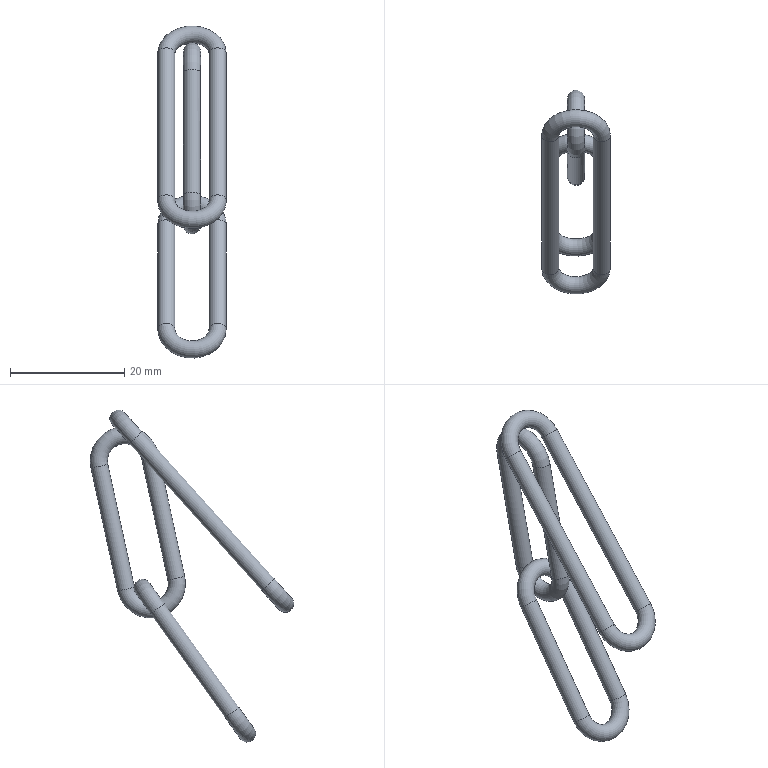Part | NX | features ACO1606-1-04.3 2 | 1 solid | 12 faces | box 12 x 35.608 x 58.107 mm | volume 1716 mm3 | torus 6 | cylinder 6 | commonest cylinder face diameters 3 x6
STEP:
#1=CARTESIAN_POINT('',(858.667,881.956,-129.86));
#2=VERTEX_POINT('',#1);
#3=CARTESIAN_POINT('',(860.167,881.956,-129.86));
#4=DIRECTION('',(0.,0.5837,0.812));
#5=DIRECTION('',(-1.,0.,0.));
#6=AXIS2_PLACEMENT_3D('',#3,#4,#5);
#7=CIRCLE('',#6,1.5);
#8=EDGE_CURVE('',#2,#2,#7,.T.);
#9=ORIENTED_EDGE('',*,*,#8,.T.);
#10=EDGE_LOOP('',(#9));
#11=FACE_BOUND('',#10,.T.);
#12=CARTESIAN_POINT('',(867.667,881.956,-129.86));
#13=VERTEX_POINT('',#12);
#14=CARTESIAN_POINT('',(869.167,881.956,-129.86));
#15=DIRECTION('',(0.,-0.5837,-0.812));
#16=DIRECTION('',(-1.,0.,0.));
#17=AXIS2_PLACEMENT_3D('',#14,#15,#16);
#18=CIRCLE('',#17,1.5);
#19=EDGE_CURVE('',#13,#13,#18,.T.);
#20=ORIENTED_EDGE('',*,*,#19,.F.);
#21=EDGE_LOOP('',(#20));
#22=FACE_BOUND('',#21,.T.);
#23=CARTESIAN_POINT('',(864.161,886.066,-126.148));
#24=VERTEX_POINT('',#23);
#25=CARTESIAN_POINT('',(865.173,886.066,-126.148));
#26=VERTEX_POINT('',#25);
#27=CARTESIAN_POINT('',(864.161,886.066,-126.148));
#28=CARTESIAN_POINT('',(863.968,886.07,-126.457));
#29=CARTESIAN_POINT('',(863.879,885.934,-127.03));
#30=CARTESIAN_POINT('',(864.124,885.389,-127.515));
#31=CARTESIAN_POINT('',(864.664,885.138,-127.587));
#32=CARTESIAN_POINT('',(865.206,885.384,-127.517));
#33=CARTESIAN_POINT('',(865.456,885.931,-127.036));
#34=CARTESIAN_POINT('',(865.366,886.07,-126.457));
#35=CARTESIAN_POINT('',(865.173,886.066,-126.148));
#36=B_SPLINE_CURVE_WITH_KNOTS('',3,(#27,#28,#29,#30,#31,#32,#33,#34,#35),.UNSPECIFIED.,.F.,.F.,(4,1,1,1,1,1,4),(-0.002168,-0.001085,-0.000544,-0.0000027,0.0005386,0.00108,0.002162),.UNSPECIFIED.);
#37=EDGE_CURVE('',#24,#26,#36,.T.);
#38=ORIENTED_EDGE('',*,*,#37,.T.);
#39=CARTESIAN_POINT('',(865.173,886.066,-126.148));
#40=CARTESIAN_POINT('',(865.064,886.064,-125.974));
#41=CARTESIAN_POINT('',(864.667,886.016,-125.734));
#42=CARTESIAN_POINT('',(864.27,886.064,-125.974));
#43=CARTESIAN_POINT('',(864.161,886.066,-126.148));
#44=B_SPLINE_CURVE_WITH_KNOTS('',3,(#39,#40,#41,#42,#43),.UNSPECIFIED.,.F.,.F.,(4,1,4),(-0.0006085,-0.000000009,0.0006085),.UNSPECIFIED.);
#45=EDGE_CURVE('',#26,#24,#44,.T.);
#46=ORIENTED_EDGE('',*,*,#45,.T.);
#47=EDGE_LOOP('',(#38,#46));
#48=FACE_BOUND('',#47,.T.);
#49=CARTESIAN_POINT('',(864.667,881.956,-129.86));
#50=DIRECTION('',(0.,0.812,-0.5837));
#51=DIRECTION('',(0.,0.5837,0.812));
#52=AXIS2_PLACEMENT_3D('',#49,#50,#51);
#53=TOROIDAL_SURFACE('',#52,4.5,1.5);
#54=ADVANCED_FACE('',(#11,#22,#48),#53,.T.);
#55=CARTESIAN_POINT('',(867.667,868.886,-148.041));
#56=VERTEX_POINT('',#55);
#57=CARTESIAN_POINT('',(869.167,868.886,-148.041));
#58=DIRECTION('',(0.,-0.5837,-0.812));
#59=DIRECTION('',(-1.,0.,0.));
#60=AXIS2_PLACEMENT_3D('',#57,#58,#59);
#61=CIRCLE('',#60,1.5);
#62=EDGE_CURVE('',#56,#56,#61,.T.);
#63=ORIENTED_EDGE('',*,*,#62,.F.);
#64=EDGE_LOOP('',(#63));
#65=FACE_BOUND('',#64,.T.);
#66=ORIENTED_EDGE('',*,*,#19,.T.);
#67=EDGE_LOOP('',(#66));
#68=FACE_BOUND('',#67,.T.);
#69=CARTESIAN_POINT('',(869.167,875.421,-138.951));
#70=DIRECTION('',(0.,0.5837,0.812));
#71=DIRECTION('',(0.,-0.812,0.5837));
#72=AXIS2_PLACEMENT_3D('',#69,#70,#71);
#73=CYLINDRICAL_SURFACE('',#72,1.5);
#74=ADVANCED_FACE('',(#65,#68),#73,.T.);
#75=ORIENTED_EDGE('',*,*,#62,.T.);
#76=EDGE_LOOP('',(#75));
#77=FACE_BOUND('',#76,.T.);
#78=CARTESIAN_POINT('',(858.667,868.886,-148.041));
#79=VERTEX_POINT('',#78);
#80=CARTESIAN_POINT('',(860.167,868.886,-148.041));
#81=DIRECTION('',(0.,0.5837,0.812));
#82=DIRECTION('',(-1.,0.,0.));
#83=AXIS2_PLACEMENT_3D('',#80,#81,#82);
#84=CIRCLE('',#83,1.5);
#85=EDGE_CURVE('',#79,#79,#84,.T.);
#86=ORIENTED_EDGE('',*,*,#85,.F.);
#87=EDGE_LOOP('',(#86));
#88=FACE_BOUND('',#87,.T.);
#89=CARTESIAN_POINT('',(864.667,868.886,-148.041));
#90=DIRECTION('',(0.,0.812,-0.5837));
#91=DIRECTION('',(0.,0.5837,0.812));
#92=AXIS2_PLACEMENT_3D('',#89,#90,#91);
#93=TOROIDAL_SURFACE('',#92,4.5,1.5);
#94=ADVANCED_FACE('',(#77,#88),#93,.T.);
#95=ORIENTED_EDGE('',*,*,#8,.F.);
#96=EDGE_LOOP('',(#95));
#97=FACE_BOUND('',#96,.T.);
#98=ORIENTED_EDGE('',*,*,#85,.T.);
#99=EDGE_LOOP('',(#98));
#100=FACE_BOUND('',#99,.T.);
#101=CARTESIAN_POINT('',(860.167,875.421,-138.951));
#102=DIRECTION('',(0.,-0.5837,-0.812));
#103=DIRECTION('',(0.,0.812,-0.5837));
#104=AXIS2_PLACEMENT_3D('',#101,#102,#103);
#105=CYLINDRICAL_SURFACE('',#104,1.5);
#106=ADVANCED_FACE('',(#97,#100),#105,.T.);
#107=CARTESIAN_POINT('',(867.667,885.762,-99.932));
#108=VERTEX_POINT('',#107);
#109=CARTESIAN_POINT('',(869.167,885.762,-99.932));
#110=DIRECTION('',(0.,0.6691,0.7431));
#111=DIRECTION('',(-1.,0.,0.));
#112=AXIS2_PLACEMENT_3D('',#109,#110,#111);
#113=CIRCLE('',#112,1.5);
#114=EDGE_CURVE('',#108,#108,#113,.T.);
#115=ORIENTED_EDGE('',*,*,#114,.T.);
#116=EDGE_LOOP('',(#115));
#117=FACE_BOUND('',#116,.T.);
#118=CARTESIAN_POINT('',(858.667,885.762,-99.932));
#119=VERTEX_POINT('',#118);
#120=CARTESIAN_POINT('',(860.167,885.762,-99.932));
#121=DIRECTION('',(0.,-0.6691,-0.7431));
#122=DIRECTION('',(-1.,0.,0.));
#123=AXIS2_PLACEMENT_3D('',#120,#121,#122);
#124=CIRCLE('',#123,1.5);
#125=EDGE_CURVE('',#119,#119,#124,.T.);
#126=ORIENTED_EDGE('',*,*,#125,.F.);
#127=EDGE_LOOP('',(#126));
#128=FACE_BOUND('',#127,.T.);
#129=CARTESIAN_POINT('',(864.667,888.765,-98.088));
#130=VERTEX_POINT('',#129);
#131=CARTESIAN_POINT('',(864.226,888.545,-98.107));
#132=CARTESIAN_POINT('',(864.667,888.875,-98.078));
#133=CARTESIAN_POINT('',(865.107,888.547,-98.108));
#134=CARTESIAN_POINT('',(864.668,888.259,-97.989));
#135=CARTESIAN_POINT('',(864.226,888.545,-98.107));
#136=CARTESIAN_POINT('',(864.667,888.875,-98.078));
#137=CARTESIAN_POINT('',(865.107,888.547,-98.108));
#138=B_SPLINE_CURVE_WITH_KNOTS('',3,(#131,#132,#133,#134,#135,#136,#137),.UNSPECIFIED.,.T.,.F.,(1,1,1,1,1,1,1,1,1,1,1),(-0.001184,-0.0007892,-0.0003946,0.,0.0003946,0.0007892,0.001184,0.001578,0.001973,0.002368,0.002762),.UNSPECIFIED.);
#139=EDGE_CURVE('',#130,#130,#138,.T.);
#140=ORIENTED_EDGE('',*,*,#139,.F.);
#141=EDGE_LOOP('',(#140));
#142=FACE_BOUND('',#141,.T.);
#143=CARTESIAN_POINT('',(864.667,885.762,-99.932));
#144=DIRECTION('',(0.,-0.7431,0.6691));
#145=DIRECTION('',(0.,-0.6691,-0.7431));
#146=AXIS2_PLACEMENT_3D('',#143,#144,#145);
#147=TOROIDAL_SURFACE('',#146,4.5,1.5);
#148=ADVANCED_FACE('',(#117,#128,#142),#147,.T.);
#149=CARTESIAN_POINT('',(858.667,862.604,-125.651));
#150=VERTEX_POINT('',#149);
#151=CARTESIAN_POINT('',(860.167,862.604,-125.651));
#152=DIRECTION('',(0.,-0.6691,-0.7431));
#153=DIRECTION('',(-1.,0.,0.));
#154=AXIS2_PLACEMENT_3D('',#151,#152,#153);
#155=CIRCLE('',#154,1.5);
#156=EDGE_CURVE('',#150,#150,#155,.T.);
#157=ORIENTED_EDGE('',*,*,#156,.F.);
#158=EDGE_LOOP('',(#157));
#159=FACE_BOUND('',#158,.T.);
#160=ORIENTED_EDGE('',*,*,#125,.T.);
#161=EDGE_LOOP('',(#160));
#162=FACE_BOUND('',#161,.T.);
#163=CARTESIAN_POINT('',(860.167,874.183,-112.791));
#164=DIRECTION('',(0.,0.6691,0.7431));
#165=DIRECTION('',(0.,-0.7431,0.6691));
#166=AXIS2_PLACEMENT_3D('',#163,#164,#165);
#167=CYLINDRICAL_SURFACE('',#166,1.5);
#168=ADVANCED_FACE('',(#159,#162),#167,.T.);
#169=ORIENTED_EDGE('',*,*,#114,.F.);
#170=EDGE_LOOP('',(#169));
#171=FACE_BOUND('',#170,.T.);
#172=CARTESIAN_POINT('',(867.667,862.604,-125.651));
#173=VERTEX_POINT('',#172);
#174=CARTESIAN_POINT('',(869.167,862.604,-125.651));
#175=DIRECTION('',(0.,0.6691,0.7431));
#176=DIRECTION('',(-1.,0.,0.));
#177=AXIS2_PLACEMENT_3D('',#174,#175,#176);
#178=CIRCLE('',#177,1.5);
#179=EDGE_CURVE('',#173,#173,#178,.T.);
#180=ORIENTED_EDGE('',*,*,#179,.T.);
#181=EDGE_LOOP('',(#180));
#182=FACE_BOUND('',#181,.T.);
#183=CARTESIAN_POINT('',(869.167,874.183,-112.791));
#184=DIRECTION('',(0.,-0.6691,-0.7431));
#185=DIRECTION('',(0.,0.7431,-0.6691));
#186=AXIS2_PLACEMENT_3D('',#183,#184,#185);
#187=CYLINDRICAL_SURFACE('',#186,1.5);
#188=ADVANCED_FACE('',(#171,#182),#187,.T.);
#189=CARTESIAN_POINT('',(863.167,883.303,-103.041));
#190=VERTEX_POINT('',#189);
#191=CARTESIAN_POINT('',(864.667,881.837,-102.724));
#192=VERTEX_POINT('',#191);
#193=CARTESIAN_POINT('',(864.667,883.303,-103.041));
#194=DIRECTION('',(0.,0.2115,0.9774));
#195=DIRECTION('',(-1.,0.,0.));
#196=AXIS2_PLACEMENT_3D('',#193,#194,#195);
#197=CIRCLE('',#196,1.5);
#198=EDGE_CURVE('',#190,#192,#197,.T.);
#199=ORIENTED_EDGE('',*,*,#198,.T.);
#200=CARTESIAN_POINT('',(866.167,883.303,-103.041));
#201=VERTEX_POINT('',#200);
#202=CARTESIAN_POINT('',(864.667,883.303,-103.041));
#203=DIRECTION('',(0.,0.2115,0.9774));
#204=DIRECTION('',(-1.,0.,0.));
#205=AXIS2_PLACEMENT_3D('',#202,#203,#204);
#206=CIRCLE('',#205,1.5);
#207=EDGE_CURVE('',#192,#201,#206,.T.);
#208=ORIENTED_EDGE('',*,*,#207,.T.);
#209=CARTESIAN_POINT('',(864.667,884.769,-103.358));
#210=VERTEX_POINT('',#209);
#211=CARTESIAN_POINT('',(864.667,883.303,-103.041));
#212=DIRECTION('',(0.,0.2115,0.9774));
#213=DIRECTION('',(-1.,0.,0.));
#214=AXIS2_PLACEMENT_3D('',#211,#212,#213);
#215=CIRCLE('',#214,1.5);
#216=EDGE_CURVE('',#201,#210,#215,.T.);
#217=ORIENTED_EDGE('',*,*,#216,.T.);
#218=CARTESIAN_POINT('',(864.667,883.303,-103.041));
#219=DIRECTION('',(0.,0.2115,0.9774));
#220=DIRECTION('',(-1.,0.,0.));
#221=AXIS2_PLACEMENT_3D('',#218,#219,#220);
#222=CIRCLE('',#221,1.5);
#223=EDGE_CURVE('',#210,#190,#222,.T.);
#224=ORIENTED_EDGE('',*,*,#223,.T.);
#225=EDGE_LOOP('',(#199,#208,#217,#224));
#226=FACE_BOUND('',#225,.T.);
#227=ORIENTED_EDGE('',*,*,#139,.T.);
#228=EDGE_LOOP('',(#227));
#229=FACE_BOUND('',#228,.T.);
#230=CARTESIAN_POINT('',(864.667,890.633,-104.627));
#231=VERTEX_POINT('',#230);
#232=CARTESIAN_POINT('',(864.667,893.565,-105.261));
#233=VERTEX_POINT('',#232);
#234=CARTESIAN_POINT('',(864.667,892.099,-104.944));
#235=DIRECTION('',(0.,-0.2115,-0.9774));
#236=DIRECTION('',(-1.,0.,0.));
#237=AXIS2_PLACEMENT_3D('',#234,#235,#236);
#238=CIRCLE('',#237,1.5);
#239=EDGE_CURVE('',#231,#233,#238,.T.);
#240=ORIENTED_EDGE('',*,*,#239,.F.);
#241=CARTESIAN_POINT('',(866.167,892.099,-104.944));
#242=VERTEX_POINT('',#241);
#243=CARTESIAN_POINT('',(864.667,892.099,-104.944));
#244=DIRECTION('',(0.,-0.2115,-0.9774));
#245=DIRECTION('',(-1.,0.,0.));
#246=AXIS2_PLACEMENT_3D('',#243,#244,#245);
#247=CIRCLE('',#246,1.5);
#248=EDGE_CURVE('',#242,#231,#247,.T.);
#249=ORIENTED_EDGE('',*,*,#248,.F.);
#250=CARTESIAN_POINT('',(864.667,892.099,-104.944));
#251=DIRECTION('',(0.,-0.2115,-0.9774));
#252=DIRECTION('',(-1.,0.,0.));
#253=AXIS2_PLACEMENT_3D('',#250,#251,#252);
#254=CIRCLE('',#253,1.5);
#255=EDGE_CURVE('',#233,#242,#254,.T.);
#256=ORIENTED_EDGE('',*,*,#255,.F.);
#257=EDGE_LOOP('',(#240,#249,#256));
#258=FACE_BOUND('',#257,.T.);
#259=CARTESIAN_POINT('',(864.667,887.701,-103.993));
#260=DIRECTION('',(-1.,0.,0.));
#261=DIRECTION('',(0.,0.,-1.));
#262=AXIS2_PLACEMENT_3D('',#259,#260,#261);
#263=TOROIDAL_SURFACE('',#262,4.5,1.5);
#264=ADVANCED_FACE('',(#226,#229,#258),#263,.T.);
#265=ORIENTED_EDGE('',*,*,#156,.T.);
#266=EDGE_LOOP('',(#265));
#267=FACE_BOUND('',#266,.T.);
#268=ORIENTED_EDGE('',*,*,#179,.F.);
#269=EDGE_LOOP('',(#268));
#270=FACE_BOUND('',#269,.T.);
#271=CARTESIAN_POINT('',(864.667,862.604,-125.651));
#272=DIRECTION('',(0.,-0.7431,0.6691));
#273=DIRECTION('',(0.,-0.6691,-0.7431));
#274=AXIS2_PLACEMENT_3D('',#271,#272,#273);
#275=TOROIDAL_SURFACE('',#274,4.5,1.5);
#276=ADVANCED_FACE('',(#267,#270),#275,.T.);
#277=ORIENTED_EDGE('',*,*,#239,.T.);
#278=ORIENTED_EDGE('',*,*,#255,.T.);
#279=ORIENTED_EDGE('',*,*,#248,.T.);
#280=EDGE_LOOP('',(#277,#278,#279));
#281=FACE_BOUND('',#280,.T.);
#282=CARTESIAN_POINT('',(864.667,887.447,-126.447));
#283=DIRECTION('',(0.,-0.2115,-0.9774));
#284=DIRECTION('',(-1.,0.,0.));
#285=AXIS2_PLACEMENT_3D('',#282,#283,#284);
#286=CIRCLE('',#285,1.5);
#287=EDGE_CURVE('',#24,#26,#286,.T.);
#288=ORIENTED_EDGE('',*,*,#287,.F.);
#289=ORIENTED_EDGE('',*,*,#45,.F.);
#290=EDGE_LOOP('',(#288,#289));
#291=FACE_BOUND('',#290,.T.);
#292=CARTESIAN_POINT('',(864.667,889.979,-114.744));
#293=DIRECTION('',(0.,-0.2115,-0.9774));
#294=DIRECTION('',(0.,0.9774,-0.2115));
#295=AXIS2_PLACEMENT_3D('',#292,#293,#294);
#296=CYLINDRICAL_SURFACE('',#295,1.5);
#297=ADVANCED_FACE('',(#281,#291),#296,.T.);
#298=CARTESIAN_POINT('',(863.167,878.65,-124.543));
#299=VERTEX_POINT('',#298);
#300=CARTESIAN_POINT('',(864.667,878.65,-124.543));
#301=DIRECTION('',(0.,0.2115,0.9774));
#302=DIRECTION('',(-1.,0.,0.));
#303=AXIS2_PLACEMENT_3D('',#300,#301,#302);
#304=CIRCLE('',#303,1.5);
#305=EDGE_CURVE('',#299,#299,#304,.T.);
#306=ORIENTED_EDGE('',*,*,#305,.T.);
#307=EDGE_LOOP('',(#306));
#308=FACE_BOUND('',#307,.T.);
#309=ORIENTED_EDGE('',*,*,#207,.F.);
#310=ORIENTED_EDGE('',*,*,#198,.F.);
#311=ORIENTED_EDGE('',*,*,#223,.F.);
#312=ORIENTED_EDGE('',*,*,#216,.F.);
#313=EDGE_LOOP('',(#309,#310,#311,#312));
#314=FACE_BOUND('',#313,.T.);
#315=CARTESIAN_POINT('',(864.667,880.77,-114.744));
#316=DIRECTION('',(0.,0.2115,0.9774));
#317=DIRECTION('',(0.,-0.9774,0.2115));
#318=AXIS2_PLACEMENT_3D('',#315,#316,#317);
#319=CYLINDRICAL_SURFACE('',#318,1.5);
#320=ADVANCED_FACE('',(#308,#314),#319,.T.);
#321=ORIENTED_EDGE('',*,*,#287,.T.);
#322=ORIENTED_EDGE('',*,*,#37,.F.);
#323=EDGE_LOOP('',(#321,#322));
#324=FACE_BOUND('',#323,.T.);
#325=ORIENTED_EDGE('',*,*,#305,.F.);
#326=EDGE_LOOP('',(#325));
#327=FACE_BOUND('',#326,.T.);
#328=CARTESIAN_POINT('',(864.667,883.048,-125.495));
#329=DIRECTION('',(-1.,0.,0.));
#330=DIRECTION('',(0.,0.,-1.));
#331=AXIS2_PLACEMENT_3D('',#328,#329,#330);
#332=TOROIDAL_SURFACE('',#331,4.5,1.5);
#333=ADVANCED_FACE('',(#324,#327),#332,.T.);
#334=CLOSED_SHELL('',(#54,#74,#94,#106,#148,#168,#188,#264,#276,#297,#320,#333));
#335=MANIFOLD_SOLID_BREP('',#334);
#336=(LENGTH_UNIT()NAMED_UNIT(*)SI_UNIT(.MILLI.,.METRE.));
#337=UNCERTAINTY_MEASURE_WITH_UNIT(LENGTH_MEASURE(0.0508),#336,'','');
#338=(NAMED_UNIT(*)PLANE_ANGLE_UNIT()SI_UNIT($,.RADIAN.));
#339=(NAMED_UNIT(*)SI_UNIT($,.STERADIAN.)SOLID_ANGLE_UNIT());
#340=(GEOMETRIC_REPRESENTATION_CONTEXT(3)GLOBAL_UNCERTAINTY_ASSIGNED_CONTEXT((#337))GLOBAL_UNIT_ASSIGNED_CONTEXT((#336,#338,#339))REPRESENTATION_CONTEXT('',''));
#341=ADVANCED_BREP_SHAPE_REPRESENTATION('',(#335),#340);